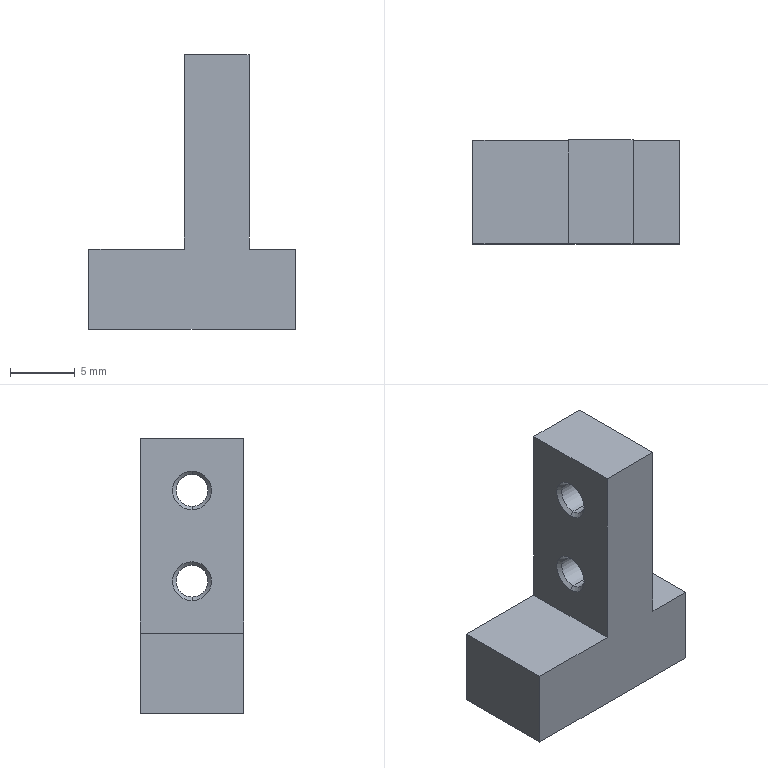Part | STEP file | 1 solid | 22 faces | box 15.9 x 8 x 21.2 mm | volume 1340 mm3 | plane 10 | cone 8 | cylinder 4 | commonest cylinder face diameters 2.46 x4
STEP:
#1=CARTESIAN_POINT('',(7.72,0.,7.53));
#2=VERTEX_POINT('',#1);
#3=CARTESIAN_POINT('',(7.72,0.,5.07));
#4=VERTEX_POINT('',#3);
#5=CARTESIAN_POINT('',(7.72,0.,6.3));
#6=DIRECTION('',(1.,0.,0.));
#7=DIRECTION('',(0.,0.,-1.));
#8=AXIS2_PLACEMENT_3D('',#5,#6,#7);
#9=CIRCLE('',#8,1.23);
#10=EDGE_CURVE('',#2,#4,#9,.T.);
#11=ORIENTED_EDGE('',*,*,#10,.F.);
#12=CARTESIAN_POINT('',(12.18,0.,7.53));
#13=VERTEX_POINT('',#12);
#14=CARTESIAN_POINT('',(6.45,0.,7.53));
#15=DIRECTION('',(1.,0.,0.));
#16=VECTOR('',#15,1000.);
#17=LINE('',#14,#16);
#18=EDGE_CURVE('',#2,#13,#17,.T.);
#19=ORIENTED_EDGE('',*,*,#18,.T.);
#20=CARTESIAN_POINT('',(12.18,0.,5.07));
#21=VERTEX_POINT('',#20);
#22=CARTESIAN_POINT('',(12.18,0.,6.3));
#23=DIRECTION('',(1.,0.,0.));
#24=DIRECTION('',(0.,0.,-1.));
#25=AXIS2_PLACEMENT_3D('',#22,#23,#24);
#26=CIRCLE('',#25,1.23);
#27=EDGE_CURVE('',#13,#21,#26,.T.);
#28=ORIENTED_EDGE('',*,*,#27,.T.);
#29=CARTESIAN_POINT('',(6.45,0.,5.07));
#30=DIRECTION('',(1.,0.,0.));
#31=VECTOR('',#30,1000.);
#32=LINE('',#29,#31);
#33=EDGE_CURVE('',#4,#21,#32,.T.);
#34=ORIENTED_EDGE('',*,*,#33,.F.);
#35=EDGE_LOOP('',(#11,#19,#28,#34));
#36=FACE_OUTER_BOUND('',#35,.T.);
#37=CARTESIAN_POINT('',(6.45,0.,6.3));
#38=DIRECTION('',(1.,0.,0.));
#39=DIRECTION('',(0.,0.,-1.));
#40=AXIS2_PLACEMENT_3D('',#37,#38,#39);
#41=CYLINDRICAL_SURFACE('',#40,1.23);
#42=ADVANCED_FACE('',(#36),#41,.F.);
#43=ORIENTED_EDGE('',*,*,#27,.F.);
#44=CARTESIAN_POINT('',(12.45,0.,7.8));
#45=VERTEX_POINT('',#44);
#46=CARTESIAN_POINT('',(12.18,0.,7.53));
#47=DIRECTION('',(0.7071,0.,0.7071));
#48=VECTOR('',#47,1000.);
#49=LINE('',#46,#48);
#50=EDGE_CURVE('',#13,#45,#49,.T.);
#51=ORIENTED_EDGE('',*,*,#50,.T.);
#52=CARTESIAN_POINT('',(12.45,0.,4.8));
#53=VERTEX_POINT('',#52);
#54=CARTESIAN_POINT('',(12.45,0.,6.3));
#55=DIRECTION('',(1.,0.,0.));
#56=DIRECTION('',(0.,0.,1.));
#57=AXIS2_PLACEMENT_3D('',#54,#55,#56);
#58=CIRCLE('',#57,1.5);
#59=EDGE_CURVE('',#45,#53,#58,.T.);
#60=ORIENTED_EDGE('',*,*,#59,.T.);
#61=CARTESIAN_POINT('',(12.18,0.,5.07));
#62=DIRECTION('',(0.7071,0.,-0.7071));
#63=VECTOR('',#62,1000.);
#64=LINE('',#61,#63);
#65=EDGE_CURVE('',#21,#53,#64,.T.);
#66=ORIENTED_EDGE('',*,*,#65,.F.);
#67=EDGE_LOOP('',(#43,#51,#60,#66));
#68=FACE_OUTER_BOUND('',#67,.T.);
#69=CARTESIAN_POINT('',(12.18,0.,6.3));
#70=DIRECTION('',(1.,0.,0.));
#71=DIRECTION('',(0.,0.,-1.));
#72=AXIS2_PLACEMENT_3D('',#69,#70,#71);
#73=CONICAL_SURFACE('',#72,1.23,0.7854);
#74=ADVANCED_FACE('',(#68),#73,.F.);
#75=ORIENTED_EDGE('',*,*,#10,.T.);
#76=CARTESIAN_POINT('',(7.45,0.,4.8));
#77=VERTEX_POINT('',#76);
#78=CARTESIAN_POINT('',(6.45,0.,3.8));
#79=DIRECTION('',(-0.7071,0.,-0.7071));
#80=VECTOR('',#79,1000.);
#81=LINE('',#78,#80);
#82=EDGE_CURVE('',#4,#77,#81,.T.);
#83=ORIENTED_EDGE('',*,*,#82,.T.);
#84=CARTESIAN_POINT('',(7.45,0.,7.8));
#85=VERTEX_POINT('',#84);
#86=CARTESIAN_POINT('',(7.45,0.,6.3));
#87=DIRECTION('',(-1.,0.,0.));
#88=DIRECTION('',(0.,0.,-1.));
#89=AXIS2_PLACEMENT_3D('',#86,#87,#88);
#90=CIRCLE('',#89,1.5);
#91=EDGE_CURVE('',#77,#85,#90,.T.);
#92=ORIENTED_EDGE('',*,*,#91,.T.);
#93=CARTESIAN_POINT('',(6.45,0.,8.8));
#94=DIRECTION('',(-0.7071,0.,0.7071));
#95=VECTOR('',#94,1000.);
#96=LINE('',#93,#95);
#97=EDGE_CURVE('',#2,#85,#96,.T.);
#98=ORIENTED_EDGE('',*,*,#97,.F.);
#99=EDGE_LOOP('',(#75,#83,#92,#98));
#100=FACE_OUTER_BOUND('',#99,.T.);
#101=CARTESIAN_POINT('',(6.45,0.,6.3));
#102=DIRECTION('',(-1.,0.,0.));
#103=DIRECTION('',(0.,0.,1.));
#104=AXIS2_PLACEMENT_3D('',#101,#102,#103);
#105=CONICAL_SURFACE('',#104,2.5,0.7854);
#106=ADVANCED_FACE('',(#100),#105,.F.);
#107=CARTESIAN_POINT('',(7.72,0.,14.53));
#108=VERTEX_POINT('',#107);
#109=CARTESIAN_POINT('',(7.72,0.,12.07));
#110=VERTEX_POINT('',#109);
#111=CARTESIAN_POINT('',(7.72,0.,13.3));
#112=DIRECTION('',(1.,0.,0.));
#113=DIRECTION('',(0.,0.,-1.));
#114=AXIS2_PLACEMENT_3D('',#111,#112,#113);
#115=CIRCLE('',#114,1.23);
#116=EDGE_CURVE('',#108,#110,#115,.T.);
#117=ORIENTED_EDGE('',*,*,#116,.F.);
#118=CARTESIAN_POINT('',(12.18,0.,14.53));
#119=VERTEX_POINT('',#118);
#120=CARTESIAN_POINT('',(6.45,0.,14.53));
#121=DIRECTION('',(1.,0.,0.));
#122=VECTOR('',#121,1000.);
#123=LINE('',#120,#122);
#124=EDGE_CURVE('',#108,#119,#123,.T.);
#125=ORIENTED_EDGE('',*,*,#124,.T.);
#126=CARTESIAN_POINT('',(12.18,0.,12.07));
#127=VERTEX_POINT('',#126);
#128=CARTESIAN_POINT('',(12.18,0.,13.3));
#129=DIRECTION('',(1.,0.,0.));
#130=DIRECTION('',(0.,0.,-1.));
#131=AXIS2_PLACEMENT_3D('',#128,#129,#130);
#132=CIRCLE('',#131,1.23);
#133=EDGE_CURVE('',#119,#127,#132,.T.);
#134=ORIENTED_EDGE('',*,*,#133,.T.);
#135=CARTESIAN_POINT('',(6.45,0.,12.07));
#136=DIRECTION('',(1.,0.,0.));
#137=VECTOR('',#136,1000.);
#138=LINE('',#135,#137);
#139=EDGE_CURVE('',#110,#127,#138,.T.);
#140=ORIENTED_EDGE('',*,*,#139,.F.);
#141=EDGE_LOOP('',(#117,#125,#134,#140));
#142=FACE_OUTER_BOUND('',#141,.T.);
#143=CARTESIAN_POINT('',(6.45,0.,13.3));
#144=DIRECTION('',(1.,0.,0.));
#145=DIRECTION('',(0.,0.,-1.));
#146=AXIS2_PLACEMENT_3D('',#143,#144,#145);
#147=CYLINDRICAL_SURFACE('',#146,1.23);
#148=ADVANCED_FACE('',(#142),#147,.F.);
#149=ORIENTED_EDGE('',*,*,#133,.F.);
#150=CARTESIAN_POINT('',(12.45,0.,14.8));
#151=VERTEX_POINT('',#150);
#152=CARTESIAN_POINT('',(12.18,0.,14.53));
#153=DIRECTION('',(0.7071,0.,0.7071));
#154=VECTOR('',#153,1000.);
#155=LINE('',#152,#154);
#156=EDGE_CURVE('',#119,#151,#155,.T.);
#157=ORIENTED_EDGE('',*,*,#156,.T.);
#158=CARTESIAN_POINT('',(12.45,0.,11.8));
#159=VERTEX_POINT('',#158);
#160=CARTESIAN_POINT('',(12.45,0.,13.3));
#161=DIRECTION('',(1.,0.,0.));
#162=DIRECTION('',(0.,0.,1.));
#163=AXIS2_PLACEMENT_3D('',#160,#161,#162);
#164=CIRCLE('',#163,1.5);
#165=EDGE_CURVE('',#151,#159,#164,.T.);
#166=ORIENTED_EDGE('',*,*,#165,.T.);
#167=CARTESIAN_POINT('',(12.18,0.,12.07));
#168=DIRECTION('',(0.7071,0.,-0.7071));
#169=VECTOR('',#168,1000.);
#170=LINE('',#167,#169);
#171=EDGE_CURVE('',#127,#159,#170,.T.);
#172=ORIENTED_EDGE('',*,*,#171,.F.);
#173=EDGE_LOOP('',(#149,#157,#166,#172));
#174=FACE_OUTER_BOUND('',#173,.T.);
#175=CARTESIAN_POINT('',(12.18,0.,13.3));
#176=DIRECTION('',(1.,0.,0.));
#177=DIRECTION('',(0.,0.,-1.));
#178=AXIS2_PLACEMENT_3D('',#175,#176,#177);
#179=CONICAL_SURFACE('',#178,1.23,0.7854);
#180=ADVANCED_FACE('',(#174),#179,.F.);
#181=ORIENTED_EDGE('',*,*,#116,.T.);
#182=CARTESIAN_POINT('',(7.45,0.,11.8));
#183=VERTEX_POINT('',#182);
#184=CARTESIAN_POINT('',(6.45,0.,10.8));
#185=DIRECTION('',(-0.7071,0.,-0.7071));
#186=VECTOR('',#185,1000.);
#187=LINE('',#184,#186);
#188=EDGE_CURVE('',#110,#183,#187,.T.);
#189=ORIENTED_EDGE('',*,*,#188,.T.);
#190=CARTESIAN_POINT('',(7.45,0.,14.8));
#191=VERTEX_POINT('',#190);
#192=CARTESIAN_POINT('',(7.45,0.,13.3));
#193=DIRECTION('',(-1.,0.,0.));
#194=DIRECTION('',(0.,0.,-1.));
#195=AXIS2_PLACEMENT_3D('',#192,#193,#194);
#196=CIRCLE('',#195,1.5);
#197=EDGE_CURVE('',#183,#191,#196,.T.);
#198=ORIENTED_EDGE('',*,*,#197,.T.);
#199=CARTESIAN_POINT('',(6.45,0.,15.8));
#200=DIRECTION('',(-0.7071,0.,0.7071));
#201=VECTOR('',#200,1000.);
#202=LINE('',#199,#201);
#203=EDGE_CURVE('',#108,#191,#202,.T.);
#204=ORIENTED_EDGE('',*,*,#203,.F.);
#205=EDGE_LOOP('',(#181,#189,#198,#204));
#206=FACE_OUTER_BOUND('',#205,.T.);
#207=CARTESIAN_POINT('',(6.45,0.,13.3));
#208=DIRECTION('',(-1.,0.,0.));
#209=DIRECTION('',(0.,0.,1.));
#210=AXIS2_PLACEMENT_3D('',#207,#208,#209);
#211=CONICAL_SURFACE('',#210,2.5,0.7854);
#212=ADVANCED_FACE('',(#206),#211,.F.);
#213=CARTESIAN_POINT('',(7.45,0.,13.3));
#214=DIRECTION('',(-1.,0.,0.));
#215=DIRECTION('',(0.,0.,-1.));
#216=AXIS2_PLACEMENT_3D('',#213,#214,#215);
#217=CIRCLE('',#216,1.5);
#218=EDGE_CURVE('',#191,#183,#217,.T.);
#219=ORIENTED_EDGE('',*,*,#218,.F.);
#220=ORIENTED_EDGE('',*,*,#197,.F.);
#221=EDGE_LOOP('',(#219,#220));
#222=FACE_BOUND('',#221,.T.);
#223=CARTESIAN_POINT('',(7.45,4.,2.3));
#224=VERTEX_POINT('',#223);
#225=CARTESIAN_POINT('',(7.45,-4.,2.3));
#226=VERTEX_POINT('',#225);
#227=CARTESIAN_POINT('',(7.45,4.,2.3));
#228=DIRECTION('',(0.,-1.,0.));
#229=VECTOR('',#228,1000.);
#230=LINE('',#227,#229);
#231=EDGE_CURVE('',#224,#226,#230,.T.);
#232=ORIENTED_EDGE('',*,*,#231,.T.);
#233=CARTESIAN_POINT('',(7.45,-4.,17.3));
#234=VERTEX_POINT('',#233);
#235=CARTESIAN_POINT('',(7.45,-4.,2.3));
#236=DIRECTION('',(0.,0.,1.));
#237=VECTOR('',#236,1000.);
#238=LINE('',#235,#237);
#239=EDGE_CURVE('',#226,#234,#238,.T.);
#240=ORIENTED_EDGE('',*,*,#239,.T.);
#241=CARTESIAN_POINT('',(7.45,4.,17.3));
#242=VERTEX_POINT('',#241);
#243=CARTESIAN_POINT('',(7.45,4.,17.3));
#244=DIRECTION('',(0.,-1.,0.));
#245=VECTOR('',#244,1000.);
#246=LINE('',#243,#245);
#247=EDGE_CURVE('',#242,#234,#246,.T.);
#248=ORIENTED_EDGE('',*,*,#247,.F.);
#249=CARTESIAN_POINT('',(7.45,4.,2.3));
#250=DIRECTION('',(0.,0.,1.));
#251=VECTOR('',#250,1000.);
#252=LINE('',#249,#251);
#253=EDGE_CURVE('',#224,#242,#252,.T.);
#254=ORIENTED_EDGE('',*,*,#253,.F.);
#255=EDGE_LOOP('',(#232,#240,#248,#254));
#256=FACE_OUTER_BOUND('',#255,.T.);
#257=CARTESIAN_POINT('',(7.45,0.,6.3));
#258=DIRECTION('',(-1.,0.,0.));
#259=DIRECTION('',(0.,0.,-1.));
#260=AXIS2_PLACEMENT_3D('',#257,#258,#259);
#261=CIRCLE('',#260,1.5);
#262=EDGE_CURVE('',#85,#77,#261,.T.);
#263=ORIENTED_EDGE('',*,*,#262,.F.);
#264=ORIENTED_EDGE('',*,*,#91,.F.);
#265=EDGE_LOOP('',(#263,#264));
#266=FACE_BOUND('',#265,.T.);
#267=CARTESIAN_POINT('',(7.45,4.,2.3));
#268=DIRECTION('',(1.,0.,0.));
#269=DIRECTION('',(0.,0.,-1.));
#270=AXIS2_PLACEMENT_3D('',#267,#268,#269);
#271=PLANE('',#270);
#272=ADVANCED_FACE('',(#222,#256,#266),#271,.F.);
#273=CARTESIAN_POINT('',(12.45,0.,13.3));
#274=DIRECTION('',(1.,0.,0.));
#275=DIRECTION('',(0.,0.,1.));
#276=AXIS2_PLACEMENT_3D('',#273,#274,#275);
#277=CIRCLE('',#276,1.5);
#278=EDGE_CURVE('',#159,#151,#277,.T.);
#279=ORIENTED_EDGE('',*,*,#278,.F.);
#280=ORIENTED_EDGE('',*,*,#165,.F.);
#281=EDGE_LOOP('',(#279,#280));
#282=FACE_BOUND('',#281,.T.);
#283=CARTESIAN_POINT('',(12.45,4.,17.3));
#284=VERTEX_POINT('',#283);
#285=CARTESIAN_POINT('',(12.45,-4.,17.3));
#286=VERTEX_POINT('',#285);
#287=CARTESIAN_POINT('',(12.45,4.,17.3));
#288=DIRECTION('',(0.,-1.,0.));
#289=VECTOR('',#288,1000.);
#290=LINE('',#287,#289);
#291=EDGE_CURVE('',#284,#286,#290,.T.);
#292=ORIENTED_EDGE('',*,*,#291,.T.);
#293=CARTESIAN_POINT('',(12.45,-4.,2.3));
#294=VERTEX_POINT('',#293);
#295=CARTESIAN_POINT('',(12.45,-4.,17.3));
#296=DIRECTION('',(0.,0.,-1.));
#297=VECTOR('',#296,1000.);
#298=LINE('',#295,#297);
#299=EDGE_CURVE('',#286,#294,#298,.T.);
#300=ORIENTED_EDGE('',*,*,#299,.T.);
#301=CARTESIAN_POINT('',(12.45,4.,2.3));
#302=VERTEX_POINT('',#301);
#303=CARTESIAN_POINT('',(12.45,4.,2.3));
#304=DIRECTION('',(0.,-1.,0.));
#305=VECTOR('',#304,1000.);
#306=LINE('',#303,#305);
#307=EDGE_CURVE('',#302,#294,#306,.T.);
#308=ORIENTED_EDGE('',*,*,#307,.F.);
#309=CARTESIAN_POINT('',(12.45,4.,17.3));
#310=DIRECTION('',(0.,0.,-1.));
#311=VECTOR('',#310,1000.);
#312=LINE('',#309,#311);
#313=EDGE_CURVE('',#284,#302,#312,.T.);
#314=ORIENTED_EDGE('',*,*,#313,.F.);
#315=EDGE_LOOP('',(#292,#300,#308,#314));
#316=FACE_OUTER_BOUND('',#315,.T.);
#317=CARTESIAN_POINT('',(12.45,0.,6.3));
#318=DIRECTION('',(1.,0.,0.));
#319=DIRECTION('',(0.,0.,1.));
#320=AXIS2_PLACEMENT_3D('',#317,#318,#319);
#321=CIRCLE('',#320,1.5);
#322=EDGE_CURVE('',#53,#45,#321,.T.);
#323=ORIENTED_EDGE('',*,*,#322,.F.);
#324=ORIENTED_EDGE('',*,*,#59,.F.);
#325=EDGE_LOOP('',(#323,#324));
#326=FACE_BOUND('',#325,.T.);
#327=CARTESIAN_POINT('',(12.45,4.,17.3));
#328=DIRECTION('',(-1.,0.,0.));
#329=DIRECTION('',(0.,0.,1.));
#330=AXIS2_PLACEMENT_3D('',#327,#328,#329);
#331=PLANE('',#330);
#332=ADVANCED_FACE('',(#282,#316,#326),#331,.F.);
#333=CARTESIAN_POINT('',(0.1,4.,-3.9));
#334=VERTEX_POINT('',#333);
#335=CARTESIAN_POINT('',(0.1,-4.,-3.9));
#336=VERTEX_POINT('',#335);
#337=CARTESIAN_POINT('',(0.1,4.,-3.9));
#338=DIRECTION('',(0.,-1.,0.));
#339=VECTOR('',#338,1000.);
#340=LINE('',#337,#339);
#341=EDGE_CURVE('',#334,#336,#340,.T.);
#342=ORIENTED_EDGE('',*,*,#341,.T.);
#343=CARTESIAN_POINT('',(0.1,-4.,2.3));
#344=VERTEX_POINT('',#343);
#345=CARTESIAN_POINT('',(0.1,-4.,-3.9));
#346=DIRECTION('',(0.,0.,1.));
#347=VECTOR('',#346,1000.);
#348=LINE('',#345,#347);
#349=EDGE_CURVE('',#336,#344,#348,.T.);
#350=ORIENTED_EDGE('',*,*,#349,.T.);
#351=CARTESIAN_POINT('',(0.1,4.,2.3));
#352=VERTEX_POINT('',#351);
#353=CARTESIAN_POINT('',(0.1,4.,2.3));
#354=DIRECTION('',(0.,-1.,0.));
#355=VECTOR('',#354,1000.);
#356=LINE('',#353,#355);
#357=EDGE_CURVE('',#352,#344,#356,.T.);
#358=ORIENTED_EDGE('',*,*,#357,.F.);
#359=CARTESIAN_POINT('',(0.1,4.,-3.9));
#360=DIRECTION('',(0.,0.,1.));
#361=VECTOR('',#360,1000.);
#362=LINE('',#359,#361);
#363=EDGE_CURVE('',#334,#352,#362,.T.);
#364=ORIENTED_EDGE('',*,*,#363,.F.);
#365=EDGE_LOOP('',(#342,#350,#358,#364));
#366=FACE_OUTER_BOUND('',#365,.T.);
#367=CARTESIAN_POINT('',(0.1,4.,-3.9));
#368=DIRECTION('',(1.,0.,0.));
#369=DIRECTION('',(0.,0.,-1.));
#370=AXIS2_PLACEMENT_3D('',#367,#368,#369);
#371=PLANE('',#370);
#372=ADVANCED_FACE('',(#366),#371,.F.);
#373=ORIENTED_EDGE('',*,*,#357,.T.);
#374=CARTESIAN_POINT('',(0.1,-4.,2.3));
#375=DIRECTION('',(1.,0.,0.));
#376=VECTOR('',#375,1000.);
#377=LINE('',#374,#376);
#378=EDGE_CURVE('',#344,#226,#377,.T.);
#379=ORIENTED_EDGE('',*,*,#378,.T.);
#380=ORIENTED_EDGE('',*,*,#231,.F.);
#381=CARTESIAN_POINT('',(0.1,4.,2.3));
#382=DIRECTION('',(1.,0.,0.));
#383=VECTOR('',#382,1000.);
#384=LINE('',#381,#383);
#385=EDGE_CURVE('',#352,#224,#384,.T.);
#386=ORIENTED_EDGE('',*,*,#385,.F.);
#387=EDGE_LOOP('',(#373,#379,#380,#386));
#388=FACE_OUTER_BOUND('',#387,.T.);
#389=CARTESIAN_POINT('',(0.1,4.,2.3));
#390=DIRECTION('',(0.,0.,-1.));
#391=DIRECTION('',(-1.,0.,0.));
#392=AXIS2_PLACEMENT_3D('',#389,#390,#391);
#393=PLANE('',#392);
#394=ADVANCED_FACE('',(#388),#393,.F.);
#395=ORIENTED_EDGE('',*,*,#247,.T.);
#396=CARTESIAN_POINT('',(7.45,-4.,17.3));
#397=DIRECTION('',(1.,0.,0.));
#398=VECTOR('',#397,1000.);
#399=LINE('',#396,#398);
#400=EDGE_CURVE('',#234,#286,#399,.T.);
#401=ORIENTED_EDGE('',*,*,#400,.T.);
#402=ORIENTED_EDGE('',*,*,#291,.F.);
#403=CARTESIAN_POINT('',(7.45,4.,17.3));
#404=DIRECTION('',(1.,0.,0.));
#405=VECTOR('',#404,1000.);
#406=LINE('',#403,#405);
#407=EDGE_CURVE('',#242,#284,#406,.T.);
#408=ORIENTED_EDGE('',*,*,#407,.F.);
#409=EDGE_LOOP('',(#395,#401,#402,#408));
#410=FACE_OUTER_BOUND('',#409,.T.);
#411=CARTESIAN_POINT('',(7.45,4.,17.3));
#412=DIRECTION('',(0.,0.,-1.));
#413=DIRECTION('',(-1.,0.,0.));
#414=AXIS2_PLACEMENT_3D('',#411,#412,#413);
#415=PLANE('',#414);
#416=ADVANCED_FACE('',(#410),#415,.F.);
#417=ORIENTED_EDGE('',*,*,#307,.T.);
#418=CARTESIAN_POINT('',(16.,-4.,2.3));
#419=VERTEX_POINT('',#418);
#420=CARTESIAN_POINT('',(12.45,-4.,2.3));
#421=DIRECTION('',(1.,0.,0.));
#422=VECTOR('',#421,1000.);
#423=LINE('',#420,#422);
#424=EDGE_CURVE('',#294,#419,#423,.T.);
#425=ORIENTED_EDGE('',*,*,#424,.T.);
#426=CARTESIAN_POINT('',(16.,4.,2.3));
#427=VERTEX_POINT('',#426);
#428=CARTESIAN_POINT('',(16.,4.,2.3));
#429=DIRECTION('',(0.,-1.,0.));
#430=VECTOR('',#429,1000.);
#431=LINE('',#428,#430);
#432=EDGE_CURVE('',#427,#419,#431,.T.);
#433=ORIENTED_EDGE('',*,*,#432,.F.);
#434=CARTESIAN_POINT('',(12.45,4.,2.3));
#435=DIRECTION('',(1.,0.,0.));
#436=VECTOR('',#435,1000.);
#437=LINE('',#434,#436);
#438=EDGE_CURVE('',#302,#427,#437,.T.);
#439=ORIENTED_EDGE('',*,*,#438,.F.);
#440=EDGE_LOOP('',(#417,#425,#433,#439));
#441=FACE_OUTER_BOUND('',#440,.T.);
#442=CARTESIAN_POINT('',(12.45,4.,2.3));
#443=DIRECTION('',(0.,0.,-1.));
#444=DIRECTION('',(-1.,0.,0.));
#445=AXIS2_PLACEMENT_3D('',#442,#443,#444);
#446=PLANE('',#445);
#447=ADVANCED_FACE('',(#441),#446,.F.);
#448=ORIENTED_EDGE('',*,*,#432,.T.);
#449=CARTESIAN_POINT('',(16.,-4.,-3.9));
#450=VERTEX_POINT('',#449);
#451=CARTESIAN_POINT('',(16.,-4.,2.3));
#452=DIRECTION('',(0.,0.,-1.));
#453=VECTOR('',#452,1000.);
#454=LINE('',#451,#453);
#455=EDGE_CURVE('',#419,#450,#454,.T.);
#456=ORIENTED_EDGE('',*,*,#455,.T.);
#457=CARTESIAN_POINT('',(16.,4.,-3.9));
#458=VERTEX_POINT('',#457);
#459=CARTESIAN_POINT('',(16.,4.,-3.9));
#460=DIRECTION('',(0.,-1.,0.));
#461=VECTOR('',#460,1000.);
#462=LINE('',#459,#461);
#463=EDGE_CURVE('',#458,#450,#462,.T.);
#464=ORIENTED_EDGE('',*,*,#463,.F.);
#465=CARTESIAN_POINT('',(16.,4.,2.3));
#466=DIRECTION('',(0.,0.,-1.));
#467=VECTOR('',#466,1000.);
#468=LINE('',#465,#467);
#469=EDGE_CURVE('',#427,#458,#468,.T.);
#470=ORIENTED_EDGE('',*,*,#469,.F.);
#471=EDGE_LOOP('',(#448,#456,#464,#470));
#472=FACE_OUTER_BOUND('',#471,.T.);
#473=CARTESIAN_POINT('',(16.,4.,2.3));
#474=DIRECTION('',(-1.,0.,0.));
#475=DIRECTION('',(0.,0.,1.));
#476=AXIS2_PLACEMENT_3D('',#473,#474,#475);
#477=PLANE('',#476);
#478=ADVANCED_FACE('',(#472),#477,.F.);
#479=ORIENTED_EDGE('',*,*,#463,.T.);
#480=CARTESIAN_POINT('',(16.,-4.,-3.9));
#481=DIRECTION('',(-1.,0.,0.));
#482=VECTOR('',#481,1000.);
#483=LINE('',#480,#482);
#484=EDGE_CURVE('',#450,#336,#483,.T.);
#485=ORIENTED_EDGE('',*,*,#484,.T.);
#486=ORIENTED_EDGE('',*,*,#341,.F.);
#487=CARTESIAN_POINT('',(16.,4.,-3.9));
#488=DIRECTION('',(-1.,0.,0.));
#489=VECTOR('',#488,1000.);
#490=LINE('',#487,#489);
#491=EDGE_CURVE('',#458,#334,#490,.T.);
#492=ORIENTED_EDGE('',*,*,#491,.F.);
#493=EDGE_LOOP('',(#479,#485,#486,#492));
#494=FACE_OUTER_BOUND('',#493,.T.);
#495=CARTESIAN_POINT('',(16.,4.,-3.9));
#496=DIRECTION('',(0.,0.,1.));
#497=DIRECTION('',(1.,0.,0.));
#498=AXIS2_PLACEMENT_3D('',#495,#496,#497);
#499=PLANE('',#498);
#500=ADVANCED_FACE('',(#494),#499,.F.);
#501=ORIENTED_EDGE('',*,*,#363,.T.);
#502=ORIENTED_EDGE('',*,*,#385,.T.);
#503=ORIENTED_EDGE('',*,*,#253,.T.);
#504=ORIENTED_EDGE('',*,*,#407,.T.);
#505=ORIENTED_EDGE('',*,*,#313,.T.);
#506=ORIENTED_EDGE('',*,*,#438,.T.);
#507=ORIENTED_EDGE('',*,*,#469,.T.);
#508=ORIENTED_EDGE('',*,*,#491,.T.);
#509=EDGE_LOOP('',(#501,#502,#503,#504,#505,#506,#507,#508));
#510=FACE_OUTER_BOUND('',#509,.T.);
#511=CARTESIAN_POINT('',(0.1,4.,2.3));
#512=DIRECTION('',(0.,1.,0.));
#513=DIRECTION('',(0.,0.,1.));
#514=AXIS2_PLACEMENT_3D('',#511,#512,#513);
#515=PLANE('',#514);
#516=ADVANCED_FACE('',(#510),#515,.T.);
#517=ORIENTED_EDGE('',*,*,#349,.F.);
#518=ORIENTED_EDGE('',*,*,#484,.F.);
#519=ORIENTED_EDGE('',*,*,#455,.F.);
#520=ORIENTED_EDGE('',*,*,#424,.F.);
#521=ORIENTED_EDGE('',*,*,#299,.F.);
#522=ORIENTED_EDGE('',*,*,#400,.F.);
#523=ORIENTED_EDGE('',*,*,#239,.F.);
#524=ORIENTED_EDGE('',*,*,#378,.F.);
#525=EDGE_LOOP('',(#517,#518,#519,#520,#521,#522,#523,#524));
#526=FACE_OUTER_BOUND('',#525,.T.);
#527=CARTESIAN_POINT('',(0.1,-4.,2.3));
#528=DIRECTION('',(0.,1.,0.));
#529=DIRECTION('',(0.,0.,1.));
#530=AXIS2_PLACEMENT_3D('',#527,#528,#529);
#531=PLANE('',#530);
#532=ADVANCED_FACE('',(#526),#531,.F.);
#533=ORIENTED_EDGE('',*,*,#188,.F.);
#534=CARTESIAN_POINT('',(7.72,0.,13.3));
#535=DIRECTION('',(1.,0.,0.));
#536=DIRECTION('',(0.,0.,-1.));
#537=AXIS2_PLACEMENT_3D('',#534,#535,#536);
#538=CIRCLE('',#537,1.23);
#539=EDGE_CURVE('',#110,#108,#538,.T.);
#540=ORIENTED_EDGE('',*,*,#539,.T.);
#541=ORIENTED_EDGE('',*,*,#203,.T.);
#542=ORIENTED_EDGE('',*,*,#218,.T.);
#543=EDGE_LOOP('',(#533,#540,#541,#542));
#544=FACE_OUTER_BOUND('',#543,.T.);
#545=CARTESIAN_POINT('',(6.45,0.,13.3));
#546=DIRECTION('',(-1.,0.,0.));
#547=DIRECTION('',(0.,0.,1.));
#548=AXIS2_PLACEMENT_3D('',#545,#546,#547);
#549=CONICAL_SURFACE('',#548,2.5,0.7854);
#550=ADVANCED_FACE('',(#544),#549,.F.);
#551=ORIENTED_EDGE('',*,*,#156,.F.);
#552=CARTESIAN_POINT('',(12.18,0.,13.3));
#553=DIRECTION('',(1.,0.,0.));
#554=DIRECTION('',(0.,0.,-1.));
#555=AXIS2_PLACEMENT_3D('',#552,#553,#554);
#556=CIRCLE('',#555,1.23);
#557=EDGE_CURVE('',#127,#119,#556,.T.);
#558=ORIENTED_EDGE('',*,*,#557,.F.);
#559=ORIENTED_EDGE('',*,*,#171,.T.);
#560=ORIENTED_EDGE('',*,*,#278,.T.);
#561=EDGE_LOOP('',(#551,#558,#559,#560));
#562=FACE_OUTER_BOUND('',#561,.T.);
#563=CARTESIAN_POINT('',(12.18,0.,13.3));
#564=DIRECTION('',(1.,0.,0.));
#565=DIRECTION('',(0.,0.,-1.));
#566=AXIS2_PLACEMENT_3D('',#563,#564,#565);
#567=CONICAL_SURFACE('',#566,1.23,0.7854);
#568=ADVANCED_FACE('',(#562),#567,.F.);
#569=ORIENTED_EDGE('',*,*,#124,.F.);
#570=ORIENTED_EDGE('',*,*,#539,.F.);
#571=ORIENTED_EDGE('',*,*,#139,.T.);
#572=ORIENTED_EDGE('',*,*,#557,.T.);
#573=EDGE_LOOP('',(#569,#570,#571,#572));
#574=FACE_OUTER_BOUND('',#573,.T.);
#575=CARTESIAN_POINT('',(6.45,0.,13.3));
#576=DIRECTION('',(1.,0.,0.));
#577=DIRECTION('',(0.,0.,-1.));
#578=AXIS2_PLACEMENT_3D('',#575,#576,#577);
#579=CYLINDRICAL_SURFACE('',#578,1.23);
#580=ADVANCED_FACE('',(#574),#579,.F.);
#581=ORIENTED_EDGE('',*,*,#82,.F.);
#582=CARTESIAN_POINT('',(7.72,0.,6.3));
#583=DIRECTION('',(1.,0.,0.));
#584=DIRECTION('',(0.,0.,-1.));
#585=AXIS2_PLACEMENT_3D('',#582,#583,#584);
#586=CIRCLE('',#585,1.23);
#587=EDGE_CURVE('',#4,#2,#586,.T.);
#588=ORIENTED_EDGE('',*,*,#587,.T.);
#589=ORIENTED_EDGE('',*,*,#97,.T.);
#590=ORIENTED_EDGE('',*,*,#262,.T.);
#591=EDGE_LOOP('',(#581,#588,#589,#590));
#592=FACE_OUTER_BOUND('',#591,.T.);
#593=CARTESIAN_POINT('',(6.45,0.,6.3));
#594=DIRECTION('',(-1.,0.,0.));
#595=DIRECTION('',(0.,0.,1.));
#596=AXIS2_PLACEMENT_3D('',#593,#594,#595);
#597=CONICAL_SURFACE('',#596,2.5,0.7854);
#598=ADVANCED_FACE('',(#592),#597,.F.);
#599=ORIENTED_EDGE('',*,*,#50,.F.);
#600=CARTESIAN_POINT('',(12.18,0.,6.3));
#601=DIRECTION('',(1.,0.,0.));
#602=DIRECTION('',(0.,0.,-1.));
#603=AXIS2_PLACEMENT_3D('',#600,#601,#602);
#604=CIRCLE('',#603,1.23);
#605=EDGE_CURVE('',#21,#13,#604,.T.);
#606=ORIENTED_EDGE('',*,*,#605,.F.);
#607=ORIENTED_EDGE('',*,*,#65,.T.);
#608=ORIENTED_EDGE('',*,*,#322,.T.);
#609=EDGE_LOOP('',(#599,#606,#607,#608));
#610=FACE_OUTER_BOUND('',#609,.T.);
#611=CARTESIAN_POINT('',(12.18,0.,6.3));
#612=DIRECTION('',(1.,0.,0.));
#613=DIRECTION('',(0.,0.,-1.));
#614=AXIS2_PLACEMENT_3D('',#611,#612,#613);
#615=CONICAL_SURFACE('',#614,1.23,0.7854);
#616=ADVANCED_FACE('',(#610),#615,.F.);
#617=ORIENTED_EDGE('',*,*,#18,.F.);
#618=ORIENTED_EDGE('',*,*,#587,.F.);
#619=ORIENTED_EDGE('',*,*,#33,.T.);
#620=ORIENTED_EDGE('',*,*,#605,.T.);
#621=EDGE_LOOP('',(#617,#618,#619,#620));
#622=FACE_OUTER_BOUND('',#621,.T.);
#623=CARTESIAN_POINT('',(6.45,0.,6.3));
#624=DIRECTION('',(1.,0.,0.));
#625=DIRECTION('',(0.,0.,-1.));
#626=AXIS2_PLACEMENT_3D('',#623,#624,#625);
#627=CYLINDRICAL_SURFACE('',#626,1.23);
#628=ADVANCED_FACE('',(#622),#627,.F.);
#629=CLOSED_SHELL('',(#42,#74,#106,#148,#180,#212,#272,#332,#372,#394,#416,#447,#478,#500,#516,#532,#550,#568,#580,#598,#616,#628));
#630=MANIFOLD_SOLID_BREP('',#629);
#631=CARTESIAN_POINT('',(0.,0.,0.));
#632=DIRECTION('',(0.,0.,1.));
#633=DIRECTION('',(1.,0.,0.));
#634=AXIS2_PLACEMENT_3D('',#631,#632,#633);
#635=(LENGTH_UNIT()NAMED_UNIT(*)SI_UNIT(.MILLI.,.METRE.));
#636=UNCERTAINTY_MEASURE_WITH_UNIT(LENGTH_MEASURE(0.00001),#635,'','');
#637=(NAMED_UNIT(*)PLANE_ANGLE_UNIT()SI_UNIT($,.RADIAN.));
#638=(NAMED_UNIT(*)SI_UNIT($,.STERADIAN.)SOLID_ANGLE_UNIT());
#639=(GEOMETRIC_REPRESENTATION_CONTEXT(3)GLOBAL_UNCERTAINTY_ASSIGNED_CONTEXT((#636))GLOBAL_UNIT_ASSIGNED_CONTEXT((#635,#637,#638))REPRESENTATION_CONTEXT('',''));
#640=ADVANCED_BREP_SHAPE_REPRESENTATION('',(#630,#634),#639);